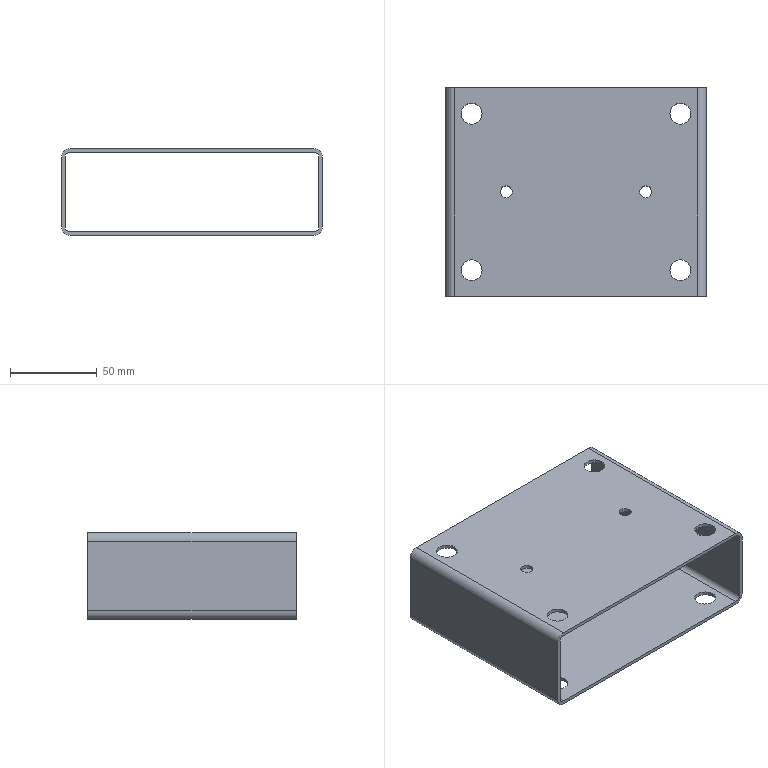Part | STEP file | Seat bracket-10P30 | 1 solid | 42 faces | box 150 x 120 x 50 mm | volume 90314 mm3 | cylinder 32 | plane 10 | commonest cylinder face diameters 12 x16 7 x8 6 x4 10 x4